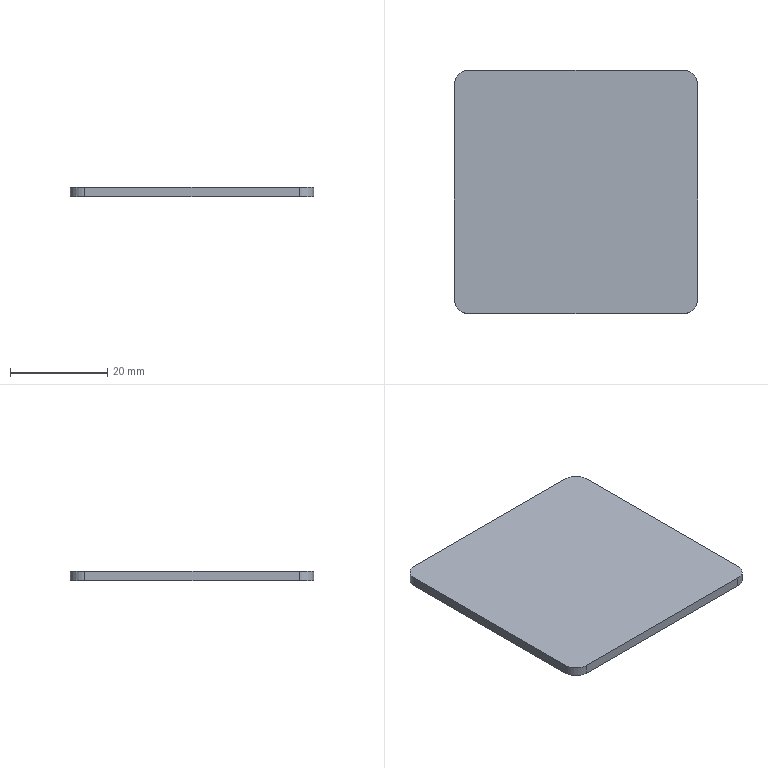Part | NX | features solid 2 | 1 solid | 10 faces | box 50 x 50 x 2 mm | volume 4985 mm3 | plane 6 | cylinder 4 | commonest cylinder face diameters 6 x4
STEP:
#1=CARTESIAN_POINT('',(1060.,47.,-605.));
#2=VERTEX_POINT('',#1);
#3=CARTESIAN_POINT('',(1063.,50.,-605.));
#4=VERTEX_POINT('',#3);
#5=CARTESIAN_POINT('',(1063.,47.,-605.));
#6=DIRECTION('',(0.,0.,-1.));
#7=DIRECTION('',(0.,1.,0.));
#8=AXIS2_PLACEMENT_3D('',#5,#6,#7);
#9=CIRCLE('',#8,3.);
#10=EDGE_CURVE('',#2,#4,#9,.T.);
#11=ORIENTED_EDGE('',*,*,#10,.F.);
#12=CARTESIAN_POINT('',(1060.,47.,-603.));
#13=VERTEX_POINT('',#12);
#14=CARTESIAN_POINT('',(1060.,47.,-605.));
#15=DIRECTION('',(0.,0.,-1.));
#16=VECTOR('',#15,1000.);
#17=LINE('',#14,#16);
#18=EDGE_CURVE('',#13,#2,#17,.T.);
#19=ORIENTED_EDGE('',*,*,#18,.F.);
#20=CARTESIAN_POINT('',(1063.,50.,-603.));
#21=VERTEX_POINT('',#20);
#22=CARTESIAN_POINT('',(1063.,47.,-603.));
#23=DIRECTION('',(0.,0.,1.));
#24=DIRECTION('',(0.,1.,0.));
#25=AXIS2_PLACEMENT_3D('',#22,#23,#24);
#26=CIRCLE('',#25,3.);
#27=EDGE_CURVE('',#21,#13,#26,.T.);
#28=ORIENTED_EDGE('',*,*,#27,.F.);
#29=CARTESIAN_POINT('',(1063.,50.,-605.));
#30=DIRECTION('',(0.,0.,1.));
#31=VECTOR('',#30,1000.);
#32=LINE('',#29,#31);
#33=EDGE_CURVE('',#4,#21,#32,.T.);
#34=ORIENTED_EDGE('',*,*,#33,.F.);
#35=EDGE_LOOP('',(#11,#19,#28,#34));
#36=FACE_BOUND('',#35,.T.);
#37=CARTESIAN_POINT('',(1063.,47.,-605.));
#38=DIRECTION('',(0.,0.,1.));
#39=DIRECTION('',(0.,1.,0.));
#40=AXIS2_PLACEMENT_3D('',#37,#38,#39);
#41=CYLINDRICAL_SURFACE('',#40,3.);
#42=ADVANCED_FACE('',(#36),#41,.T.);
#43=CARTESIAN_POINT('',(1063.,0.,-605.));
#44=VERTEX_POINT('',#43);
#45=CARTESIAN_POINT('',(1060.,3.,-605.));
#46=VERTEX_POINT('',#45);
#47=CARTESIAN_POINT('',(1063.,3.,-605.));
#48=DIRECTION('',(0.,0.,-1.));
#49=DIRECTION('',(0.,1.,0.));
#50=AXIS2_PLACEMENT_3D('',#47,#48,#49);
#51=CIRCLE('',#50,3.);
#52=EDGE_CURVE('',#44,#46,#51,.T.);
#53=ORIENTED_EDGE('',*,*,#52,.F.);
#54=CARTESIAN_POINT('',(1063.,0.,-603.));
#55=VERTEX_POINT('',#54);
#56=CARTESIAN_POINT('',(1063.,0.,-605.));
#57=DIRECTION('',(0.,0.,-1.));
#58=VECTOR('',#57,1000.);
#59=LINE('',#56,#58);
#60=EDGE_CURVE('',#55,#44,#59,.T.);
#61=ORIENTED_EDGE('',*,*,#60,.F.);
#62=CARTESIAN_POINT('',(1060.,3.,-603.));
#63=VERTEX_POINT('',#62);
#64=CARTESIAN_POINT('',(1063.,3.,-603.));
#65=DIRECTION('',(0.,0.,1.));
#66=DIRECTION('',(0.,1.,0.));
#67=AXIS2_PLACEMENT_3D('',#64,#65,#66);
#68=CIRCLE('',#67,3.);
#69=EDGE_CURVE('',#63,#55,#68,.T.);
#70=ORIENTED_EDGE('',*,*,#69,.F.);
#71=CARTESIAN_POINT('',(1060.,3.,-605.));
#72=DIRECTION('',(0.,0.,1.));
#73=VECTOR('',#72,1000.);
#74=LINE('',#71,#73);
#75=EDGE_CURVE('',#46,#63,#74,.T.);
#76=ORIENTED_EDGE('',*,*,#75,.F.);
#77=EDGE_LOOP('',(#53,#61,#70,#76));
#78=FACE_BOUND('',#77,.T.);
#79=CARTESIAN_POINT('',(1063.,3.,-605.));
#80=DIRECTION('',(0.,0.,1.));
#81=DIRECTION('',(0.,1.,0.));
#82=AXIS2_PLACEMENT_3D('',#79,#80,#81);
#83=CYLINDRICAL_SURFACE('',#82,3.);
#84=ADVANCED_FACE('',(#78),#83,.T.);
#85=CARTESIAN_POINT('',(1110.,3.,-605.));
#86=VERTEX_POINT('',#85);
#87=CARTESIAN_POINT('',(1107.,0.,-605.));
#88=VERTEX_POINT('',#87);
#89=CARTESIAN_POINT('',(1107.,3.,-605.));
#90=DIRECTION('',(0.,0.,-1.));
#91=DIRECTION('',(0.,1.,0.));
#92=AXIS2_PLACEMENT_3D('',#89,#90,#91);
#93=CIRCLE('',#92,3.);
#94=EDGE_CURVE('',#86,#88,#93,.T.);
#95=ORIENTED_EDGE('',*,*,#94,.F.);
#96=CARTESIAN_POINT('',(1110.,3.,-603.));
#97=VERTEX_POINT('',#96);
#98=CARTESIAN_POINT('',(1110.,3.,-605.));
#99=DIRECTION('',(0.,0.,-1.));
#100=VECTOR('',#99,1000.);
#101=LINE('',#98,#100);
#102=EDGE_CURVE('',#97,#86,#101,.T.);
#103=ORIENTED_EDGE('',*,*,#102,.F.);
#104=CARTESIAN_POINT('',(1107.,0.,-603.));
#105=VERTEX_POINT('',#104);
#106=CARTESIAN_POINT('',(1107.,3.,-603.));
#107=DIRECTION('',(0.,0.,1.));
#108=DIRECTION('',(0.,1.,0.));
#109=AXIS2_PLACEMENT_3D('',#106,#107,#108);
#110=CIRCLE('',#109,3.);
#111=EDGE_CURVE('',#105,#97,#110,.T.);
#112=ORIENTED_EDGE('',*,*,#111,.F.);
#113=CARTESIAN_POINT('',(1107.,0.,-605.));
#114=DIRECTION('',(0.,0.,1.));
#115=VECTOR('',#114,1000.);
#116=LINE('',#113,#115);
#117=EDGE_CURVE('',#88,#105,#116,.T.);
#118=ORIENTED_EDGE('',*,*,#117,.F.);
#119=EDGE_LOOP('',(#95,#103,#112,#118));
#120=FACE_BOUND('',#119,.T.);
#121=CARTESIAN_POINT('',(1107.,3.,-605.));
#122=DIRECTION('',(0.,0.,1.));
#123=DIRECTION('',(0.,1.,0.));
#124=AXIS2_PLACEMENT_3D('',#121,#122,#123);
#125=CYLINDRICAL_SURFACE('',#124,3.);
#126=ADVANCED_FACE('',(#120),#125,.T.);
#127=CARTESIAN_POINT('',(1107.,50.,-605.));
#128=VERTEX_POINT('',#127);
#129=CARTESIAN_POINT('',(1110.,47.,-605.));
#130=VERTEX_POINT('',#129);
#131=CARTESIAN_POINT('',(1107.,47.,-605.));
#132=DIRECTION('',(0.,0.,-1.));
#133=DIRECTION('',(0.,1.,0.));
#134=AXIS2_PLACEMENT_3D('',#131,#132,#133);
#135=CIRCLE('',#134,3.);
#136=EDGE_CURVE('',#128,#130,#135,.T.);
#137=ORIENTED_EDGE('',*,*,#136,.F.);
#138=CARTESIAN_POINT('',(1107.,50.,-603.));
#139=VERTEX_POINT('',#138);
#140=CARTESIAN_POINT('',(1107.,50.,-605.));
#141=DIRECTION('',(0.,0.,-1.));
#142=VECTOR('',#141,1000.);
#143=LINE('',#140,#142);
#144=EDGE_CURVE('',#139,#128,#143,.T.);
#145=ORIENTED_EDGE('',*,*,#144,.F.);
#146=CARTESIAN_POINT('',(1110.,47.,-603.));
#147=VERTEX_POINT('',#146);
#148=CARTESIAN_POINT('',(1107.,47.,-603.));
#149=DIRECTION('',(0.,0.,1.));
#150=DIRECTION('',(0.,1.,0.));
#151=AXIS2_PLACEMENT_3D('',#148,#149,#150);
#152=CIRCLE('',#151,3.);
#153=EDGE_CURVE('',#147,#139,#152,.T.);
#154=ORIENTED_EDGE('',*,*,#153,.F.);
#155=CARTESIAN_POINT('',(1110.,47.,-605.));
#156=DIRECTION('',(0.,0.,1.));
#157=VECTOR('',#156,1000.);
#158=LINE('',#155,#157);
#159=EDGE_CURVE('',#130,#147,#158,.T.);
#160=ORIENTED_EDGE('',*,*,#159,.F.);
#161=EDGE_LOOP('',(#137,#145,#154,#160));
#162=FACE_BOUND('',#161,.T.);
#163=CARTESIAN_POINT('',(1107.,47.,-605.));
#164=DIRECTION('',(0.,0.,1.));
#165=DIRECTION('',(0.,1.,0.));
#166=AXIS2_PLACEMENT_3D('',#163,#164,#165);
#167=CYLINDRICAL_SURFACE('',#166,3.);
#168=ADVANCED_FACE('',(#162),#167,.T.);
#169=CARTESIAN_POINT('',(1110.,0.,-603.));
#170=DIRECTION('',(0.,1.,0.));
#171=VECTOR('',#170,1000.);
#172=LINE('',#169,#171);
#173=EDGE_CURVE('',#97,#147,#172,.T.);
#174=ORIENTED_EDGE('',*,*,#173,.T.);
#175=ORIENTED_EDGE('',*,*,#153,.T.);
#176=CARTESIAN_POINT('',(1060.,50.,-603.));
#177=DIRECTION('',(-1.,0.,0.));
#178=VECTOR('',#177,1000.);
#179=LINE('',#176,#178);
#180=EDGE_CURVE('',#139,#21,#179,.T.);
#181=ORIENTED_EDGE('',*,*,#180,.T.);
#182=ORIENTED_EDGE('',*,*,#27,.T.);
#183=CARTESIAN_POINT('',(1060.,0.,-603.));
#184=DIRECTION('',(0.,-1.,0.));
#185=VECTOR('',#184,1000.);
#186=LINE('',#183,#185);
#187=EDGE_CURVE('',#13,#63,#186,.T.);
#188=ORIENTED_EDGE('',*,*,#187,.T.);
#189=ORIENTED_EDGE('',*,*,#69,.T.);
#190=CARTESIAN_POINT('',(1060.,0.,-603.));
#191=DIRECTION('',(1.,0.,0.));
#192=VECTOR('',#191,1000.);
#193=LINE('',#190,#192);
#194=EDGE_CURVE('',#55,#105,#193,.T.);
#195=ORIENTED_EDGE('',*,*,#194,.T.);
#196=ORIENTED_EDGE('',*,*,#111,.T.);
#197=EDGE_LOOP('',(#174,#175,#181,#182,#188,#189,#195,#196));
#198=FACE_BOUND('',#197,.T.);
#199=CARTESIAN_POINT('',(1126.005,1.443,-603.));
#200=DIRECTION('',(0.,0.,1.));
#201=DIRECTION('',(0.,-1.,0.));
#202=AXIS2_PLACEMENT_3D('',#199,#200,#201);
#203=PLANE('',#202);
#204=ADVANCED_FACE('',(#198),#203,.T.);
#205=CARTESIAN_POINT('',(1060.,50.,-605.));
#206=DIRECTION('',(-1.,0.,0.));
#207=VECTOR('',#206,1000.);
#208=LINE('',#205,#207);
#209=EDGE_CURVE('',#128,#4,#208,.T.);
#210=ORIENTED_EDGE('',*,*,#209,.F.);
#211=ORIENTED_EDGE('',*,*,#136,.T.);
#212=CARTESIAN_POINT('',(1110.,0.,-605.));
#213=DIRECTION('',(0.,1.,0.));
#214=VECTOR('',#213,1000.);
#215=LINE('',#212,#214);
#216=EDGE_CURVE('',#86,#130,#215,.T.);
#217=ORIENTED_EDGE('',*,*,#216,.F.);
#218=ORIENTED_EDGE('',*,*,#94,.T.);
#219=CARTESIAN_POINT('',(1060.,0.,-605.));
#220=DIRECTION('',(1.,0.,0.));
#221=VECTOR('',#220,1000.);
#222=LINE('',#219,#221);
#223=EDGE_CURVE('',#44,#88,#222,.T.);
#224=ORIENTED_EDGE('',*,*,#223,.F.);
#225=ORIENTED_EDGE('',*,*,#52,.T.);
#226=CARTESIAN_POINT('',(1060.,0.,-605.));
#227=DIRECTION('',(0.,-1.,0.));
#228=VECTOR('',#227,1000.);
#229=LINE('',#226,#228);
#230=EDGE_CURVE('',#2,#46,#229,.T.);
#231=ORIENTED_EDGE('',*,*,#230,.F.);
#232=ORIENTED_EDGE('',*,*,#10,.T.);
#233=EDGE_LOOP('',(#210,#211,#217,#218,#224,#225,#231,#232));
#234=FACE_BOUND('',#233,.T.);
#235=CARTESIAN_POINT('',(1126.005,1.443,-605.));
#236=DIRECTION('',(0.,0.,1.));
#237=DIRECTION('',(0.,-1.,0.));
#238=AXIS2_PLACEMENT_3D('',#235,#236,#237);
#239=PLANE('',#238);
#240=ADVANCED_FACE('',(#234),#239,.F.);
#241=ORIENTED_EDGE('',*,*,#230,.T.);
#242=ORIENTED_EDGE('',*,*,#75,.T.);
#243=ORIENTED_EDGE('',*,*,#187,.F.);
#244=ORIENTED_EDGE('',*,*,#18,.T.);
#245=EDGE_LOOP('',(#241,#242,#243,#244));
#246=FACE_BOUND('',#245,.T.);
#247=CARTESIAN_POINT('',(1060.,0.,-605.));
#248=DIRECTION('',(-1.,0.,0.));
#249=DIRECTION('',(0.,0.,1.));
#250=AXIS2_PLACEMENT_3D('',#247,#248,#249);
#251=PLANE('',#250);
#252=ADVANCED_FACE('',(#246),#251,.T.);
#253=ORIENTED_EDGE('',*,*,#180,.F.);
#254=ORIENTED_EDGE('',*,*,#144,.T.);
#255=ORIENTED_EDGE('',*,*,#209,.T.);
#256=ORIENTED_EDGE('',*,*,#33,.T.);
#257=EDGE_LOOP('',(#253,#254,#255,#256));
#258=FACE_BOUND('',#257,.T.);
#259=CARTESIAN_POINT('',(1060.,50.,-605.));
#260=DIRECTION('',(0.,1.,0.));
#261=DIRECTION('',(1.,0.,0.));
#262=AXIS2_PLACEMENT_3D('',#259,#260,#261);
#263=PLANE('',#262);
#264=ADVANCED_FACE('',(#258),#263,.T.);
#265=ORIENTED_EDGE('',*,*,#216,.T.);
#266=ORIENTED_EDGE('',*,*,#159,.T.);
#267=ORIENTED_EDGE('',*,*,#173,.F.);
#268=ORIENTED_EDGE('',*,*,#102,.T.);
#269=EDGE_LOOP('',(#265,#266,#267,#268));
#270=FACE_BOUND('',#269,.T.);
#271=CARTESIAN_POINT('',(1110.,0.,-605.));
#272=DIRECTION('',(1.,0.,0.));
#273=DIRECTION('',(0.,-1.,0.));
#274=AXIS2_PLACEMENT_3D('',#271,#272,#273);
#275=PLANE('',#274);
#276=ADVANCED_FACE('',(#270),#275,.T.);
#277=ORIENTED_EDGE('',*,*,#223,.T.);
#278=ORIENTED_EDGE('',*,*,#117,.T.);
#279=ORIENTED_EDGE('',*,*,#194,.F.);
#280=ORIENTED_EDGE('',*,*,#60,.T.);
#281=EDGE_LOOP('',(#277,#278,#279,#280));
#282=FACE_BOUND('',#281,.T.);
#283=CARTESIAN_POINT('',(1060.,0.,-605.));
#284=DIRECTION('',(0.,-1.,0.));
#285=DIRECTION('',(-1.,0.,0.));
#286=AXIS2_PLACEMENT_3D('',#283,#284,#285);
#287=PLANE('',#286);
#288=ADVANCED_FACE('',(#282),#287,.T.);
#289=CLOSED_SHELL('',(#42,#84,#126,#168,#204,#240,#252,#264,#276,#288));
#290=MANIFOLD_SOLID_BREP('',#289);
#291=(LENGTH_UNIT()NAMED_UNIT(*)SI_UNIT(.MILLI.,.METRE.));
#292=UNCERTAINTY_MEASURE_WITH_UNIT(LENGTH_MEASURE(0.00001),#291,'','');
#293=(NAMED_UNIT(*)PLANE_ANGLE_UNIT()SI_UNIT($,.RADIAN.));
#294=(NAMED_UNIT(*)SI_UNIT($,.STERADIAN.)SOLID_ANGLE_UNIT());
#295=(GEOMETRIC_REPRESENTATION_CONTEXT(3)GLOBAL_UNCERTAINTY_ASSIGNED_CONTEXT((#292))GLOBAL_UNIT_ASSIGNED_CONTEXT((#291,#293,#294))REPRESENTATION_CONTEXT('',''));
#296=ADVANCED_BREP_SHAPE_REPRESENTATION('',(#290),#295);